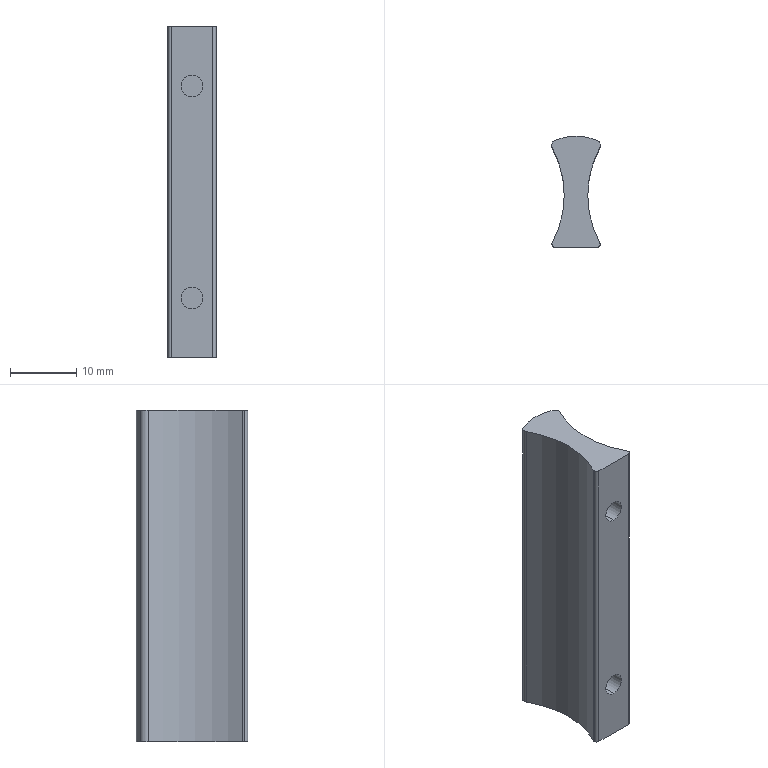Part | STEP file | TOPNIKE 1205 aluminium handle, hole spacing 32mm | 1 solid | 19 faces | box 7.369 x 16.8 x 50 mm | volume 4040 mm3 | cylinder 14 | plane 5 | commonest cylinder face diameters 3.3 x4 1 x3 1.6 x3 30 x3 16 x1
STEP:
#1=CARTESIAN_POINT('',(0.,0.,0.));
#2=DIRECTION('',(0.,0.,1.));
#3=DIRECTION('',(1.,0.,0.));
#4=AXIS2_PLACEMENT_3D('',#1,#2,#3);
#5=CARTESIAN_POINT('',(-3.634,-8.3,25.));
#6=VERTEX_POINT('',#5);
#7=CARTESIAN_POINT('',(-3.134,-8.8,25.));
#8=VERTEX_POINT('',#7);
#9=CARTESIAN_POINT('',(-3.134,-8.3,25.));
#10=DIRECTION('',(0.,0.,1.));
#11=DIRECTION('',(-1.,0.,0.));
#12=AXIS2_PLACEMENT_3D('',#9,#10,#11);
#13=CIRCLE('',#12,0.5);
#14=CARTESIAN_POINT('',(-3.134,-8.3,25.));
#15=DIRECTION('',(0.,0.,-1.));
#16=DIRECTION('',(-1.,0.,0.));
#17=AXIS2_PLACEMENT_3D('',#14,#15,#16);
#18=CYLINDRICAL_SURFACE('',#17,0.5);
#19=CARTESIAN_POINT('',(6.283,0.));
#20=DIRECTION('',(-1.,0.));
#21=VECTOR('',#20,1.);
#22=LINE('',#19,#21);
#23=(GEOMETRIC_REPRESENTATION_CONTEXT(2)PARAMETRIC_REPRESENTATION_CONTEXT()REPRESENTATION_CONTEXT('',''));
#24=DEFINITIONAL_REPRESENTATION('',(#22),#23);
#25=PCURVE('',#18,#24);
#26=CARTESIAN_POINT('',(-16.773,-0.9359,25.));
#27=DIRECTION('',(0.,0.,-1.));
#28=DIRECTION('',(-1.,0.,0.));
#29=AXIS2_PLACEMENT_3D('',#26,#27,#28);
#30=PLANE('',#29);
#31=CARTESIAN_POINT('',(-13.139,-7.364));
#32=CARTESIAN_POINT('',(-13.139,-8.23));
#33=CARTESIAN_POINT('',(-13.889,-7.797));
#34=CARTESIAN_POINT('',(-14.639,-7.364));
#35=CARTESIAN_POINT('',(-13.889,-6.931));
#36=CARTESIAN_POINT('',(-13.139,-6.498));
#37=CARTESIAN_POINT('',(-13.139,-7.364));
#38=(BOUNDED_CURVE()B_SPLINE_CURVE(2,(#31,#32,#33,#34,#35,#36,#37),.UNSPECIFIED.,.T.,.F.)B_SPLINE_CURVE_WITH_KNOTS((1,2,2,2,2,1),(-2.094,0.,2.094,4.189,6.283,8.378),.UNSPECIFIED.)CURVE()GEOMETRIC_REPRESENTATION_ITEM()RATIONAL_B_SPLINE_CURVE((1.,0.5,1.,0.5,1.,0.5,1.))REPRESENTATION_ITEM(''));
#39=(GEOMETRIC_REPRESENTATION_CONTEXT(2)PARAMETRIC_REPRESENTATION_CONTEXT()REPRESENTATION_CONTEXT('',''));
#40=DEFINITIONAL_REPRESENTATION('',(#38),#39);
#41=PCURVE('',#30,#40);
#42=SURFACE_CURVE('',#13,(#25,#41),.PCURVE_S1.);
#43=EDGE_CURVE('',#6,#8,#42,.T.);
#44=ORIENTED_EDGE('',*,*,#43,.F.);
#45=CARTESIAN_POINT('',(-3.634,-8.3,-25.));
#46=VERTEX_POINT('',#45);
#47=CARTESIAN_POINT('',(-3.634,-8.3,25.));
#48=DIRECTION('',(0.,0.,-1.));
#49=VECTOR('',#48,1.);
#50=LINE('',#47,#49);
#51=CARTESIAN_POINT('',(6.283,0.));
#52=DIRECTION('',(0.,1.));
#53=VECTOR('',#52,1.);
#54=LINE('',#51,#53);
#55=(GEOMETRIC_REPRESENTATION_CONTEXT(2)PARAMETRIC_REPRESENTATION_CONTEXT()REPRESENTATION_CONTEXT('',''));
#56=DEFINITIONAL_REPRESENTATION('',(#54),#55);
#57=PCURVE('',#18,#56);
#58=CARTESIAN_POINT('',(-3.134,-8.3,25.));
#59=DIRECTION('',(0.,0.,-1.));
#60=DIRECTION('',(-1.,0.,0.));
#61=AXIS2_PLACEMENT_3D('',#58,#59,#60);
#62=CYLINDRICAL_SURFACE('',#61,0.5);
#63=CARTESIAN_POINT('',(0.,0.));
#64=DIRECTION('',(0.,1.));
#65=VECTOR('',#64,1.);
#66=LINE('',#63,#65);
#67=(GEOMETRIC_REPRESENTATION_CONTEXT(2)PARAMETRIC_REPRESENTATION_CONTEXT()REPRESENTATION_CONTEXT('',''));
#68=DEFINITIONAL_REPRESENTATION('',(#66),#67);
#69=PCURVE('',#62,#68);
#70=SURFACE_CURVE('',#50,(#57,#69),.PCURVE_S1.);
#71=EDGE_CURVE('',#6,#46,#70,.T.);
#72=ORIENTED_EDGE('',*,*,#71,.T.);
#73=CARTESIAN_POINT('',(-3.134,-8.8,-25.));
#74=VERTEX_POINT('',#73);
#75=CARTESIAN_POINT('',(-3.134,-8.3,-25.));
#76=DIRECTION('',(0.,0.,-1.));
#77=DIRECTION('',(-1.,0.,0.));
#78=AXIS2_PLACEMENT_3D('',#75,#76,#77);
#79=CIRCLE('',#78,0.5);
#80=CARTESIAN_POINT('',(0.,50.));
#81=DIRECTION('',(1.,0.));
#82=VECTOR('',#81,1.);
#83=LINE('',#80,#82);
#84=(GEOMETRIC_REPRESENTATION_CONTEXT(2)PARAMETRIC_REPRESENTATION_CONTEXT()REPRESENTATION_CONTEXT('',''));
#85=DEFINITIONAL_REPRESENTATION('',(#83),#84);
#86=PCURVE('',#18,#85);
#87=CARTESIAN_POINT('',(-16.773,-0.9359,-25.));
#88=DIRECTION('',(0.,0.,-1.));
#89=DIRECTION('',(-1.,0.,0.));
#90=AXIS2_PLACEMENT_3D('',#87,#88,#89);
#91=PLANE('',#90);
#92=CARTESIAN_POINT('',(-13.639,-7.364));
#93=DIRECTION('',(1.,0.));
#94=AXIS2_PLACEMENT_2D('',#92,#93);
#95=CIRCLE('',#94,0.5);
#96=(GEOMETRIC_REPRESENTATION_CONTEXT(2)PARAMETRIC_REPRESENTATION_CONTEXT()REPRESENTATION_CONTEXT('',''));
#97=DEFINITIONAL_REPRESENTATION('',(#95),#96);
#98=PCURVE('',#91,#97);
#99=SURFACE_CURVE('',#79,(#86,#98),.PCURVE_S1.);
#100=EDGE_CURVE('',#74,#46,#99,.T.);
#101=ORIENTED_EDGE('',*,*,#100,.F.);
#102=CARTESIAN_POINT('',(-3.134,-8.8,25.));
#103=DIRECTION('',(0.,0.,-1.));
#104=VECTOR('',#103,1.);
#105=LINE('',#102,#104);
#106=CARTESIAN_POINT('',(4.712,0.));
#107=DIRECTION('',(0.,1.));
#108=VECTOR('',#107,1.);
#109=LINE('',#106,#108);
#110=(GEOMETRIC_REPRESENTATION_CONTEXT(2)PARAMETRIC_REPRESENTATION_CONTEXT()REPRESENTATION_CONTEXT('',''));
#111=DEFINITIONAL_REPRESENTATION('',(#109),#110);
#112=PCURVE('',#18,#111);
#113=CARTESIAN_POINT('',(4.,-8.8,25.));
#114=DIRECTION('',(0.,1.,0.));
#115=DIRECTION('',(0.,0.,1.));
#116=AXIS2_PLACEMENT_3D('',#113,#114,#115);
#117=PLANE('',#116);
#118=CARTESIAN_POINT('',(0.,-7.134));
#119=DIRECTION('',(-1.,0.));
#120=VECTOR('',#119,1.);
#121=LINE('',#118,#120);
#122=(GEOMETRIC_REPRESENTATION_CONTEXT(2)PARAMETRIC_REPRESENTATION_CONTEXT()REPRESENTATION_CONTEXT('',''));
#123=DEFINITIONAL_REPRESENTATION('',(#121),#122);
#124=PCURVE('',#117,#123);
#125=SURFACE_CURVE('',#105,(#112,#124),.PCURVE_S1.);
#126=EDGE_CURVE('',#8,#74,#125,.T.);
#127=ORIENTED_EDGE('',*,*,#126,.F.);
#128=EDGE_LOOP('',(#44,#72,#101,#127));
#129=FACE_BOUND('',#128,.T.);
#130=ADVANCED_FACE('',(#129),#18,.T.);
#131=CARTESIAN_POINT('',(3.685,6.597,-25.));
#132=VERTEX_POINT('',#131);
#133=CARTESIAN_POINT('',(3.588,6.216,-25.));
#134=VERTEX_POINT('',#133);
#135=CARTESIAN_POINT('',(2.885,6.597,-25.));
#136=DIRECTION('',(0.,0.,-1.));
#137=DIRECTION('',(-1.,0.,0.));
#138=AXIS2_PLACEMENT_3D('',#135,#136,#137);
#139=CIRCLE('',#138,0.8);
#140=CARTESIAN_POINT('',(2.885,6.597,25.));
#141=DIRECTION('',(0.,0.,1.));
#142=DIRECTION('',(1.,0.,0.));
#143=AXIS2_PLACEMENT_3D('',#140,#141,#142);
#144=CYLINDRICAL_SURFACE('',#143,0.8);
#145=CARTESIAN_POINT('',(9.425,-50.));
#146=DIRECTION('',(-1.,0.));
#147=VECTOR('',#146,1.);
#148=LINE('',#145,#147);
#149=(GEOMETRIC_REPRESENTATION_CONTEXT(2)PARAMETRIC_REPRESENTATION_CONTEXT()REPRESENTATION_CONTEXT('',''));
#150=DEFINITIONAL_REPRESENTATION('',(#148),#149);
#151=PCURVE('',#144,#150);
#152=CARTESIAN_POINT('',(-19.658,7.533));
#153=DIRECTION('',(1.,0.));
#154=AXIS2_PLACEMENT_2D('',#152,#153);
#155=CIRCLE('',#154,0.8);
#156=(GEOMETRIC_REPRESENTATION_CONTEXT(2)PARAMETRIC_REPRESENTATION_CONTEXT()REPRESENTATION_CONTEXT('',''));
#157=DEFINITIONAL_REPRESENTATION('',(#155),#156);
#158=PCURVE('',#91,#157);
#159=SURFACE_CURVE('',#139,(#151,#158),.PCURVE_S1.);
#160=EDGE_CURVE('',#132,#134,#159,.T.);
#161=ORIENTED_EDGE('',*,*,#160,.F.);
#162=CARTESIAN_POINT('',(3.685,6.597,25.));
#163=VERTEX_POINT('',#162);
#164=CARTESIAN_POINT('',(3.685,6.597,25.));
#165=DIRECTION('',(0.,0.,1.));
#166=VECTOR('',#165,1.);
#167=LINE('',#164,#166);
#168=CARTESIAN_POINT('',(6.283,0.));
#169=DIRECTION('',(0.,1.));
#170=VECTOR('',#169,1.);
#171=LINE('',#168,#170);
#172=(GEOMETRIC_REPRESENTATION_CONTEXT(2)PARAMETRIC_REPRESENTATION_CONTEXT()REPRESENTATION_CONTEXT('',''));
#173=DEFINITIONAL_REPRESENTATION('',(#171),#172);
#174=PCURVE('',#144,#173);
#175=CARTESIAN_POINT('',(2.885,6.597,25.));
#176=DIRECTION('',(0.,0.,1.));
#177=DIRECTION('',(1.,0.,0.));
#178=AXIS2_PLACEMENT_3D('',#175,#176,#177);
#179=CYLINDRICAL_SURFACE('',#178,0.8);
#180=CARTESIAN_POINT('',(0.,0.));
#181=DIRECTION('',(0.,1.));
#182=VECTOR('',#181,1.);
#183=LINE('',#180,#182);
#184=(GEOMETRIC_REPRESENTATION_CONTEXT(2)PARAMETRIC_REPRESENTATION_CONTEXT()REPRESENTATION_CONTEXT('',''));
#185=DEFINITIONAL_REPRESENTATION('',(#183),#184);
#186=PCURVE('',#179,#185);
#187=SURFACE_CURVE('',#167,(#174,#186),.PCURVE_S1.);
#188=EDGE_CURVE('',#132,#163,#187,.T.);
#189=ORIENTED_EDGE('',*,*,#188,.T.);
#190=CARTESIAN_POINT('',(3.588,6.216,25.));
#191=VERTEX_POINT('',#190);
#192=CARTESIAN_POINT('',(2.885,6.597,25.));
#193=DIRECTION('',(0.,0.,1.));
#194=DIRECTION('',(-1.,0.,0.));
#195=AXIS2_PLACEMENT_3D('',#192,#193,#194);
#196=CIRCLE('',#195,0.8);
#197=CARTESIAN_POINT('',(3.142,0.));
#198=DIRECTION('',(1.,0.));
#199=VECTOR('',#198,1.);
#200=LINE('',#197,#199);
#201=(GEOMETRIC_REPRESENTATION_CONTEXT(2)PARAMETRIC_REPRESENTATION_CONTEXT()REPRESENTATION_CONTEXT('',''));
#202=DEFINITIONAL_REPRESENTATION('',(#200),#201);
#203=PCURVE('',#144,#202);
#204=CARTESIAN_POINT('',(-18.858,7.533));
#205=CARTESIAN_POINT('',(-18.858,6.147));
#206=CARTESIAN_POINT('',(-20.058,6.84));
#207=CARTESIAN_POINT('',(-21.258,7.533));
#208=CARTESIAN_POINT('',(-20.058,8.226));
#209=CARTESIAN_POINT('',(-18.858,8.918));
#210=CARTESIAN_POINT('',(-18.858,7.533));
#211=(BOUNDED_CURVE()B_SPLINE_CURVE(2,(#204,#205,#206,#207,#208,#209,#210),.UNSPECIFIED.,.T.,.F.)B_SPLINE_CURVE_WITH_KNOTS((1,2,2,2,2,1),(-2.094,0.,2.094,4.189,6.283,8.378),.UNSPECIFIED.)CURVE()GEOMETRIC_REPRESENTATION_ITEM()RATIONAL_B_SPLINE_CURVE((1.,0.5,1.,0.5,1.,0.5,1.))REPRESENTATION_ITEM(''));
#212=(GEOMETRIC_REPRESENTATION_CONTEXT(2)PARAMETRIC_REPRESENTATION_CONTEXT()REPRESENTATION_CONTEXT('',''));
#213=DEFINITIONAL_REPRESENTATION('',(#211),#212);
#214=PCURVE('',#30,#213);
#215=SURFACE_CURVE('',#196,(#203,#214),.PCURVE_S1.);
#216=EDGE_CURVE('',#191,#163,#215,.T.);
#217=ORIENTED_EDGE('',*,*,#216,.F.);
#218=CARTESIAN_POINT('',(3.588,6.216,25.));
#219=DIRECTION('',(0.,0.,1.));
#220=VECTOR('',#219,1.);
#221=LINE('',#218,#220);
#222=CARTESIAN_POINT('',(5.786,0.));
#223=DIRECTION('',(0.,1.));
#224=VECTOR('',#223,1.);
#225=LINE('',#222,#224);
#226=(GEOMETRIC_REPRESENTATION_CONTEXT(2)PARAMETRIC_REPRESENTATION_CONTEXT()REPRESENTATION_CONTEXT('',''));
#227=DEFINITIONAL_REPRESENTATION('',(#225),#226);
#228=PCURVE('',#144,#227);
#229=CARTESIAN_POINT('',(16.773,-0.9359,25.));
#230=DIRECTION('',(0.,0.,-1.));
#231=DIRECTION('',(-1.,0.,0.));
#232=AXIS2_PLACEMENT_3D('',#229,#230,#231);
#233=CYLINDRICAL_SURFACE('',#232,15.);
#234=CARTESIAN_POINT('',(0.497,0.));
#235=DIRECTION('',(0.,-1.));
#236=VECTOR('',#235,1.);
#237=LINE('',#234,#236);
#238=(GEOMETRIC_REPRESENTATION_CONTEXT(2)PARAMETRIC_REPRESENTATION_CONTEXT()REPRESENTATION_CONTEXT('',''));
#239=DEFINITIONAL_REPRESENTATION('',(#237),#238);
#240=PCURVE('',#233,#239);
#241=SURFACE_CURVE('',#221,(#228,#240),.PCURVE_S1.);
#242=EDGE_CURVE('',#134,#191,#241,.T.);
#243=ORIENTED_EDGE('',*,*,#242,.F.);
#244=EDGE_LOOP('',(#161,#189,#217,#243));
#245=FACE_BOUND('',#244,.T.);
#246=ADVANCED_FACE('',(#245),#144,.T.);
#247=CARTESIAN_POINT('',(0.,-0.8,-17.65));
#248=VERTEX_POINT('',#247);
#249=CARTESIAN_POINT('',(0.,-8.8,-17.65));
#250=VERTEX_POINT('',#249);
#251=CARTESIAN_POINT('',(0.,-0.8,-17.65));
#252=DIRECTION('',(0.,-1.,0.));
#253=VECTOR('',#252,1.);
#254=LINE('',#251,#253);
#255=CARTESIAN_POINT('',(0.,-0.8,-16.));
#256=DIRECTION('',(0.,-1.,0.));
#257=DIRECTION('',(0.,0.,-1.));
#258=AXIS2_PLACEMENT_3D('',#255,#256,#257);
#259=CYLINDRICAL_SURFACE('',#258,1.65);
#260=CARTESIAN_POINT('',(6.283,0.));
#261=DIRECTION('',(0.,1.));
#262=VECTOR('',#261,1.);
#263=LINE('',#260,#262);
#264=(GEOMETRIC_REPRESENTATION_CONTEXT(2)PARAMETRIC_REPRESENTATION_CONTEXT()REPRESENTATION_CONTEXT('',''));
#265=DEFINITIONAL_REPRESENTATION('',(#263),#264);
#266=PCURVE('',#259,#265);
#267=CARTESIAN_POINT('',(0.,-0.8,-16.));
#268=DIRECTION('',(0.,-1.,0.));
#269=DIRECTION('',(0.,0.,-1.));
#270=AXIS2_PLACEMENT_3D('',#267,#268,#269);
#271=CYLINDRICAL_SURFACE('',#270,1.65);
#272=CARTESIAN_POINT('',(0.,0.));
#273=DIRECTION('',(0.,1.));
#274=VECTOR('',#273,1.);
#275=LINE('',#272,#274);
#276=(GEOMETRIC_REPRESENTATION_CONTEXT(2)PARAMETRIC_REPRESENTATION_CONTEXT()REPRESENTATION_CONTEXT('',''));
#277=DEFINITIONAL_REPRESENTATION('',(#275),#276);
#278=PCURVE('',#271,#277);
#279=SURFACE_CURVE('',#254,(#266,#278),.PCURVE_S1.);
#280=EDGE_CURVE('',#248,#250,#279,.T.);
#281=ORIENTED_EDGE('',*,*,#280,.T.);
#282=CARTESIAN_POINT('',(0.,-8.8,-14.35));
#283=VERTEX_POINT('',#282);
#284=CARTESIAN_POINT('',(0.,-8.8,-16.));
#285=DIRECTION('',(0.,-1.,0.));
#286=DIRECTION('',(0.,0.,-1.));
#287=AXIS2_PLACEMENT_3D('',#284,#285,#286);
#288=CIRCLE('',#287,1.65);
#289=CARTESIAN_POINT('',(0.,8.));
#290=DIRECTION('',(1.,0.));
#291=VECTOR('',#290,1.);
#292=LINE('',#289,#291);
#293=(GEOMETRIC_REPRESENTATION_CONTEXT(2)PARAMETRIC_REPRESENTATION_CONTEXT()REPRESENTATION_CONTEXT('',''));
#294=DEFINITIONAL_REPRESENTATION('',(#292),#293);
#295=PCURVE('',#259,#294);
#296=CARTESIAN_POINT('',(-42.65,-4.));
#297=CARTESIAN_POINT('',(-42.65,-1.142));
#298=CARTESIAN_POINT('',(-40.175,-2.571));
#299=CARTESIAN_POINT('',(-37.7,-4.));
#300=CARTESIAN_POINT('',(-40.175,-5.429));
#301=CARTESIAN_POINT('',(-42.65,-6.858));
#302=CARTESIAN_POINT('',(-42.65,-4.));
#303=(BOUNDED_CURVE()B_SPLINE_CURVE(2,(#296,#297,#298,#299,#300,#301,#302),.UNSPECIFIED.,.T.,.F.)B_SPLINE_CURVE_WITH_KNOTS((1,2,2,2,2,1),(-2.094,0.,2.094,4.189,6.283,8.378),.UNSPECIFIED.)CURVE()GEOMETRIC_REPRESENTATION_ITEM()RATIONAL_B_SPLINE_CURVE((1.,0.5,1.,0.5,1.,0.5,1.))REPRESENTATION_ITEM(''));
#304=(GEOMETRIC_REPRESENTATION_CONTEXT(2)PARAMETRIC_REPRESENTATION_CONTEXT()REPRESENTATION_CONTEXT('',''));
#305=DEFINITIONAL_REPRESENTATION('',(#303),#304);
#306=PCURVE('',#117,#305);
#307=SURFACE_CURVE('',#288,(#295,#306),.PCURVE_S1.);
#308=EDGE_CURVE('',#283,#250,#307,.T.);
#309=ORIENTED_EDGE('',*,*,#308,.F.);
#310=CARTESIAN_POINT('',(0.,-0.8,-14.35));
#311=VERTEX_POINT('',#310);
#312=CARTESIAN_POINT('',(0.,-0.8,-14.35));
#313=DIRECTION('',(0.,-1.,0.));
#314=VECTOR('',#313,1.);
#315=LINE('',#312,#314);
#316=CARTESIAN_POINT('',(3.142,0.));
#317=DIRECTION('',(0.,1.));
#318=VECTOR('',#317,1.);
#319=LINE('',#316,#318);
#320=(GEOMETRIC_REPRESENTATION_CONTEXT(2)PARAMETRIC_REPRESENTATION_CONTEXT()REPRESENTATION_CONTEXT('',''));
#321=DEFINITIONAL_REPRESENTATION('',(#319),#320);
#322=PCURVE('',#259,#321);
#323=CARTESIAN_POINT('',(3.142,0.));
#324=DIRECTION('',(0.,1.));
#325=VECTOR('',#324,1.);
#326=LINE('',#323,#325);
#327=(GEOMETRIC_REPRESENTATION_CONTEXT(2)PARAMETRIC_REPRESENTATION_CONTEXT()REPRESENTATION_CONTEXT('',''));
#328=DEFINITIONAL_REPRESENTATION('',(#326),#327);
#329=PCURVE('',#271,#328);
#330=SURFACE_CURVE('',#315,(#322,#329),.PCURVE_S1.);
#331=EDGE_CURVE('',#311,#283,#330,.T.);
#332=ORIENTED_EDGE('',*,*,#331,.F.);
#333=CARTESIAN_POINT('',(0.,-0.8,-16.));
#334=DIRECTION('',(0.,-1.,0.));
#335=DIRECTION('',(0.,0.,-1.));
#336=AXIS2_PLACEMENT_3D('',#333,#334,#335);
#337=CIRCLE('',#336,1.65);
#338=CARTESIAN_POINT('',(0.,0.));
#339=DIRECTION('',(1.,0.));
#340=VECTOR('',#339,1.);
#341=LINE('',#338,#340);
#342=(GEOMETRIC_REPRESENTATION_CONTEXT(2)PARAMETRIC_REPRESENTATION_CONTEXT()REPRESENTATION_CONTEXT('',''));
#343=DEFINITIONAL_REPRESENTATION('',(#341),#342);
#344=PCURVE('',#259,#343);
#345=CARTESIAN_POINT('',(0.,-0.8,-16.));
#346=DIRECTION('',(0.,-1.,0.));
#347=DIRECTION('',(0.,0.,-1.));
#348=AXIS2_PLACEMENT_3D('',#345,#346,#347);
#349=PLANE('',#348);
#350=CARTESIAN_POINT('',(0.,0.));
#351=DIRECTION('',(1.,0.));
#352=AXIS2_PLACEMENT_2D('',#350,#351);
#353=CIRCLE('',#352,1.65);
#354=(GEOMETRIC_REPRESENTATION_CONTEXT(2)PARAMETRIC_REPRESENTATION_CONTEXT()REPRESENTATION_CONTEXT('',''));
#355=DEFINITIONAL_REPRESENTATION('',(#353),#354);
#356=PCURVE('',#349,#355);
#357=SURFACE_CURVE('',#337,(#344,#356),.PCURVE_S1.);
#358=EDGE_CURVE('',#311,#248,#357,.T.);
#359=ORIENTED_EDGE('',*,*,#358,.T.);
#360=EDGE_LOOP('',(#281,#309,#332,#359));
#361=FACE_BOUND('',#360,.F.);
#362=ADVANCED_FACE('',(#361),#259,.F.);
#363=CARTESIAN_POINT('',(0.,-0.8,14.35));
#364=VERTEX_POINT('',#363);
#365=CARTESIAN_POINT('',(0.,-8.8,14.35));
#366=VERTEX_POINT('',#365);
#367=CARTESIAN_POINT('',(0.,-0.8,14.35));
#368=DIRECTION('',(0.,-1.,0.));
#369=VECTOR('',#368,1.);
#370=LINE('',#367,#369);
#371=CARTESIAN_POINT('',(0.,-0.8,16.));
#372=DIRECTION('',(0.,-1.,0.));
#373=DIRECTION('',(0.,0.,-1.));
#374=AXIS2_PLACEMENT_3D('',#371,#372,#373);
#375=CYLINDRICAL_SURFACE('',#374,1.65);
#376=CARTESIAN_POINT('',(6.283,0.));
#377=DIRECTION('',(0.,1.));
#378=VECTOR('',#377,1.);
#379=LINE('',#376,#378);
#380=(GEOMETRIC_REPRESENTATION_CONTEXT(2)PARAMETRIC_REPRESENTATION_CONTEXT()REPRESENTATION_CONTEXT('',''));
#381=DEFINITIONAL_REPRESENTATION('',(#379),#380);
#382=PCURVE('',#375,#381);
#383=CARTESIAN_POINT('',(0.,-0.8,16.));
#384=DIRECTION('',(0.,-1.,0.));
#385=DIRECTION('',(0.,0.,-1.));
#386=AXIS2_PLACEMENT_3D('',#383,#384,#385);
#387=CYLINDRICAL_SURFACE('',#386,1.65);
#388=CARTESIAN_POINT('',(0.,0.));
#389=DIRECTION('',(0.,1.));
#390=VECTOR('',#389,1.);
#391=LINE('',#388,#390);
#392=(GEOMETRIC_REPRESENTATION_CONTEXT(2)PARAMETRIC_REPRESENTATION_CONTEXT()REPRESENTATION_CONTEXT('',''));
#393=DEFINITIONAL_REPRESENTATION('',(#391),#392);
#394=PCURVE('',#387,#393);
#395=SURFACE_CURVE('',#370,(#382,#394),.PCURVE_S1.);
#396=EDGE_CURVE('',#364,#366,#395,.T.);
#397=ORIENTED_EDGE('',*,*,#396,.T.);
#398=CARTESIAN_POINT('',(0.,-8.8,17.65));
#399=VERTEX_POINT('',#398);
#400=CARTESIAN_POINT('',(0.,-8.8,16.));
#401=DIRECTION('',(0.,-1.,0.));
#402=DIRECTION('',(0.,0.,-1.));
#403=AXIS2_PLACEMENT_3D('',#400,#401,#402);
#404=CIRCLE('',#403,1.65);
#405=CARTESIAN_POINT('',(0.,8.));
#406=DIRECTION('',(1.,0.));
#407=VECTOR('',#406,1.);
#408=LINE('',#405,#407);
#409=(GEOMETRIC_REPRESENTATION_CONTEXT(2)PARAMETRIC_REPRESENTATION_CONTEXT()REPRESENTATION_CONTEXT('',''));
#410=DEFINITIONAL_REPRESENTATION('',(#408),#409);
#411=PCURVE('',#375,#410);
#412=CARTESIAN_POINT('',(-10.65,-4.));
#413=CARTESIAN_POINT('',(-10.65,-1.142));
#414=CARTESIAN_POINT('',(-8.175,-2.571));
#415=CARTESIAN_POINT('',(-5.7,-4.));
#416=CARTESIAN_POINT('',(-8.175,-5.429));
#417=CARTESIAN_POINT('',(-10.65,-6.858));
#418=CARTESIAN_POINT('',(-10.65,-4.));
#419=(BOUNDED_CURVE()B_SPLINE_CURVE(2,(#412,#413,#414,#415,#416,#417,#418),.UNSPECIFIED.,.T.,.F.)B_SPLINE_CURVE_WITH_KNOTS((1,2,2,2,2,1),(-2.094,0.,2.094,4.189,6.283,8.378),.UNSPECIFIED.)CURVE()GEOMETRIC_REPRESENTATION_ITEM()RATIONAL_B_SPLINE_CURVE((1.,0.5,1.,0.5,1.,0.5,1.))REPRESENTATION_ITEM(''));
#420=(GEOMETRIC_REPRESENTATION_CONTEXT(2)PARAMETRIC_REPRESENTATION_CONTEXT()REPRESENTATION_CONTEXT('',''));
#421=DEFINITIONAL_REPRESENTATION('',(#419),#420);
#422=PCURVE('',#117,#421);
#423=SURFACE_CURVE('',#404,(#411,#422),.PCURVE_S1.);
#424=EDGE_CURVE('',#399,#366,#423,.T.);
#425=ORIENTED_EDGE('',*,*,#424,.F.);
#426=CARTESIAN_POINT('',(0.,-0.8,17.65));
#427=VERTEX_POINT('',#426);
#428=CARTESIAN_POINT('',(0.,-0.8,17.65));
#429=DIRECTION('',(0.,-1.,0.));
#430=VECTOR('',#429,1.);
#431=LINE('',#428,#430);
#432=CARTESIAN_POINT('',(3.142,0.));
#433=DIRECTION('',(0.,1.));
#434=VECTOR('',#433,1.);
#435=LINE('',#432,#434);
#436=(GEOMETRIC_REPRESENTATION_CONTEXT(2)PARAMETRIC_REPRESENTATION_CONTEXT()REPRESENTATION_CONTEXT('',''));
#437=DEFINITIONAL_REPRESENTATION('',(#435),#436);
#438=PCURVE('',#375,#437);
#439=CARTESIAN_POINT('',(3.142,0.));
#440=DIRECTION('',(0.,1.));
#441=VECTOR('',#440,1.);
#442=LINE('',#439,#441);
#443=(GEOMETRIC_REPRESENTATION_CONTEXT(2)PARAMETRIC_REPRESENTATION_CONTEXT()REPRESENTATION_CONTEXT('',''));
#444=DEFINITIONAL_REPRESENTATION('',(#442),#443);
#445=PCURVE('',#387,#444);
#446=SURFACE_CURVE('',#431,(#438,#445),.PCURVE_S1.);
#447=EDGE_CURVE('',#427,#399,#446,.T.);
#448=ORIENTED_EDGE('',*,*,#447,.F.);
#449=CARTESIAN_POINT('',(0.,-0.8,16.));
#450=DIRECTION('',(0.,-1.,0.));
#451=DIRECTION('',(0.,0.,-1.));
#452=AXIS2_PLACEMENT_3D('',#449,#450,#451);
#453=CIRCLE('',#452,1.65);
#454=CARTESIAN_POINT('',(0.,0.));
#455=DIRECTION('',(1.,0.));
#456=VECTOR('',#455,1.);
#457=LINE('',#454,#456);
#458=(GEOMETRIC_REPRESENTATION_CONTEXT(2)PARAMETRIC_REPRESENTATION_CONTEXT()REPRESENTATION_CONTEXT('',''));
#459=DEFINITIONAL_REPRESENTATION('',(#457),#458);
#460=PCURVE('',#375,#459);
#461=CARTESIAN_POINT('',(0.,-0.8,16.));
#462=DIRECTION('',(0.,-1.,0.));
#463=DIRECTION('',(0.,0.,-1.));
#464=AXIS2_PLACEMENT_3D('',#461,#462,#463);
#465=PLANE('',#464);
#466=CARTESIAN_POINT('',(0.,0.));
#467=DIRECTION('',(1.,0.));
#468=AXIS2_PLACEMENT_2D('',#466,#467);
#469=CIRCLE('',#468,1.65);
#470=(GEOMETRIC_REPRESENTATION_CONTEXT(2)PARAMETRIC_REPRESENTATION_CONTEXT()REPRESENTATION_CONTEXT('',''));
#471=DEFINITIONAL_REPRESENTATION('',(#469),#470);
#472=PCURVE('',#465,#471);
#473=SURFACE_CURVE('',#453,(#460,#472),.PCURVE_S1.);
#474=EDGE_CURVE('',#427,#364,#473,.T.);
#475=ORIENTED_EDGE('',*,*,#474,.T.);
#476=EDGE_LOOP('',(#397,#425,#448,#475));
#477=FACE_BOUND('',#476,.F.);
#478=ADVANCED_FACE('',(#477),#375,.F.);
#479=ORIENTED_EDGE('',*,*,#242,.F.);
#480=CARTESIAN_POINT('',(1.773,-0.9359,-25.));
#481=VERTEX_POINT('',#480);
#482=CARTESIAN_POINT('',(16.773,-0.9359,-25.));
#483=DIRECTION('',(0.,0.,-1.));
#484=DIRECTION('',(1.,0.,0.));
#485=AXIS2_PLACEMENT_3D('',#482,#483,#484);
#486=CIRCLE('',#485,15.);
#487=CARTESIAN_POINT('',(-3.142,50.));
#488=DIRECTION('',(1.,0.));
#489=VECTOR('',#488,1.);
#490=LINE('',#487,#489);
#491=(GEOMETRIC_REPRESENTATION_CONTEXT(2)PARAMETRIC_REPRESENTATION_CONTEXT()REPRESENTATION_CONTEXT('',''));
#492=DEFINITIONAL_REPRESENTATION('',(#490),#491);
#493=PCURVE('',#233,#492);
#494=CARTESIAN_POINT('',(-33.546,0.));
#495=DIRECTION('',(-1.,0.));
#496=AXIS2_PLACEMENT_2D('',#494,#495);
#497=CIRCLE('',#496,15.);
#498=(GEOMETRIC_REPRESENTATION_CONTEXT(2)PARAMETRIC_REPRESENTATION_CONTEXT()REPRESENTATION_CONTEXT('',''));
#499=DEFINITIONAL_REPRESENTATION('',(#497),#498);
#500=PCURVE('',#91,#499);
#501=SURFACE_CURVE('',#486,(#493,#500),.PCURVE_S1.);
#502=EDGE_CURVE('',#481,#134,#501,.T.);
#503=ORIENTED_EDGE('',*,*,#502,.F.);
#504=CARTESIAN_POINT('',(1.773,-0.9359,25.));
#505=VERTEX_POINT('',#504);
#506=CARTESIAN_POINT('',(1.773,-0.9359,25.));
#507=DIRECTION('',(0.,0.,-1.));
#508=VECTOR('',#507,1.);
#509=LINE('',#506,#508);
#510=CARTESIAN_POINT('',(0.,0.));
#511=DIRECTION('',(0.,1.));
#512=VECTOR('',#511,1.);
#513=LINE('',#510,#512);
#514=(GEOMETRIC_REPRESENTATION_CONTEXT(2)PARAMETRIC_REPRESENTATION_CONTEXT()REPRESENTATION_CONTEXT('',''));
#515=DEFINITIONAL_REPRESENTATION('',(#513),#514);
#516=PCURVE('',#233,#515);
#517=CARTESIAN_POINT('',(16.773,-0.9359,25.));
#518=DIRECTION('',(0.,0.,-1.));
#519=DIRECTION('',(-1.,0.,0.));
#520=AXIS2_PLACEMENT_3D('',#517,#518,#519);
#521=CYLINDRICAL_SURFACE('',#520,15.);
#522=CARTESIAN_POINT('',(6.283,0.));
#523=DIRECTION('',(0.,1.));
#524=VECTOR('',#523,1.);
#525=LINE('',#522,#524);
#526=(GEOMETRIC_REPRESENTATION_CONTEXT(2)PARAMETRIC_REPRESENTATION_CONTEXT()REPRESENTATION_CONTEXT('',''));
#527=DEFINITIONAL_REPRESENTATION('',(#525),#526);
#528=PCURVE('',#521,#527);
#529=SURFACE_CURVE('',#509,(#516,#528),.PCURVE_S1.);
#530=EDGE_CURVE('',#505,#481,#529,.T.);
#531=ORIENTED_EDGE('',*,*,#530,.F.);
#532=CARTESIAN_POINT('',(16.773,-0.9359,25.));
#533=DIRECTION('',(0.,0.,-1.));
#534=DIRECTION('',(1.,0.,0.));
#535=AXIS2_PLACEMENT_3D('',#532,#533,#534);
#536=CIRCLE('',#535,15.);
#537=CARTESIAN_POINT('',(-3.142,0.));
#538=DIRECTION('',(1.,0.));
#539=VECTOR('',#538,1.);
#540=LINE('',#537,#539);
#541=(GEOMETRIC_REPRESENTATION_CONTEXT(2)PARAMETRIC_REPRESENTATION_CONTEXT()REPRESENTATION_CONTEXT('',''));
#542=DEFINITIONAL_REPRESENTATION('',(#540),#541);
#543=PCURVE('',#233,#542);
#544=CARTESIAN_POINT('',(-33.546,0.));
#545=DIRECTION('',(-1.,0.));
#546=AXIS2_PLACEMENT_2D('',#544,#545);
#547=CIRCLE('',#546,15.);
#548=(GEOMETRIC_REPRESENTATION_CONTEXT(2)PARAMETRIC_REPRESENTATION_CONTEXT()REPRESENTATION_CONTEXT('',''));
#549=DEFINITIONAL_REPRESENTATION('',(#547),#548);
#550=PCURVE('',#30,#549);
#551=SURFACE_CURVE('',#536,(#543,#550),.PCURVE_S1.);
#552=EDGE_CURVE('',#505,#191,#551,.T.);
#553=ORIENTED_EDGE('',*,*,#552,.T.);
#554=EDGE_LOOP('',(#479,#503,#531,#553));
#555=FACE_BOUND('',#554,.F.);
#556=ADVANCED_FACE('',(#555),#233,.F.);
#557=CARTESIAN_POINT('',(-3.588,6.216,25.));
#558=VERTEX_POINT('',#557);
#559=CARTESIAN_POINT('',(-3.588,6.216,-25.));
#560=VERTEX_POINT('',#559);
#561=CARTESIAN_POINT('',(-3.588,6.216,25.));
#562=DIRECTION('',(0.,0.,-1.));
#563=VECTOR('',#562,1.);
#564=LINE('',#561,#563);
#565=CARTESIAN_POINT('',(-16.773,-0.9359,25.));
#566=DIRECTION('',(0.,0.,-1.));
#567=DIRECTION('',(-1.,0.,0.));
#568=AXIS2_PLACEMENT_3D('',#565,#566,#567);
#569=CYLINDRICAL_SURFACE('',#568,15.);
#570=CARTESIAN_POINT('',(2.645,0.));
#571=DIRECTION('',(0.,1.));
#572=VECTOR('',#571,1.);
#573=LINE('',#570,#572);
#574=(GEOMETRIC_REPRESENTATION_CONTEXT(2)PARAMETRIC_REPRESENTATION_CONTEXT()REPRESENTATION_CONTEXT('',''));
#575=DEFINITIONAL_REPRESENTATION('',(#573),#574);
#576=PCURVE('',#569,#575);
#577=CARTESIAN_POINT('',(-2.885,6.597,25.));
#578=DIRECTION('',(0.,0.,1.));
#579=DIRECTION('',(1.,0.,0.));
#580=AXIS2_PLACEMENT_3D('',#577,#578,#579);
#581=CYLINDRICAL_SURFACE('',#580,0.8);
#582=CARTESIAN_POINT('',(3.639,0.));
#583=DIRECTION('',(0.,-1.));
#584=VECTOR('',#583,1.);
#585=LINE('',#582,#584);
#586=(GEOMETRIC_REPRESENTATION_CONTEXT(2)PARAMETRIC_REPRESENTATION_CONTEXT()REPRESENTATION_CONTEXT('',''));
#587=DEFINITIONAL_REPRESENTATION('',(#585),#586);
#588=PCURVE('',#581,#587);
#589=SURFACE_CURVE('',#564,(#576,#588),.PCURVE_S1.);
#590=EDGE_CURVE('',#558,#560,#589,.T.);
#591=ORIENTED_EDGE('',*,*,#590,.F.);
#592=CARTESIAN_POINT('',(-3.574,-8.062,25.));
#593=VERTEX_POINT('',#592);
#594=CARTESIAN_POINT('',(-16.773,-0.9359,25.));
#595=DIRECTION('',(0.,0.,-1.));
#596=DIRECTION('',(-1.,0.,0.));
#597=AXIS2_PLACEMENT_3D('',#594,#595,#596);
#598=CIRCLE('',#597,15.);
#599=CARTESIAN_POINT('',(0.,0.));
#600=DIRECTION('',(1.,0.));
#601=VECTOR('',#600,1.);
#602=LINE('',#599,#601);
#603=(GEOMETRIC_REPRESENTATION_CONTEXT(2)PARAMETRIC_REPRESENTATION_CONTEXT()REPRESENTATION_CONTEXT('',''));
#604=DEFINITIONAL_REPRESENTATION('',(#602),#603);
#605=PCURVE('',#569,#604);
#606=CARTESIAN_POINT('',(0.,0.));
#607=DIRECTION('',(1.,0.));
#608=AXIS2_PLACEMENT_2D('',#606,#607);
#609=CIRCLE('',#608,15.);
#610=(GEOMETRIC_REPRESENTATION_CONTEXT(2)PARAMETRIC_REPRESENTATION_CONTEXT()REPRESENTATION_CONTEXT('',''));
#611=DEFINITIONAL_REPRESENTATION('',(#609),#610);
#612=PCURVE('',#30,#611);
#613=SURFACE_CURVE('',#598,(#605,#612),.PCURVE_S1.);
#614=EDGE_CURVE('',#558,#593,#613,.T.);
#615=ORIENTED_EDGE('',*,*,#614,.T.);
#616=CARTESIAN_POINT('',(-3.574,-8.062,-25.));
#617=VERTEX_POINT('',#616);
#618=CARTESIAN_POINT('',(-3.574,-8.062,25.));
#619=DIRECTION('',(0.,0.,1.));
#620=VECTOR('',#619,1.);
#621=LINE('',#618,#620);
#622=CARTESIAN_POINT('',(3.637,0.));
#623=DIRECTION('',(0.,-1.));
#624=VECTOR('',#623,1.);
#625=LINE('',#622,#624);
#626=(GEOMETRIC_REPRESENTATION_CONTEXT(2)PARAMETRIC_REPRESENTATION_CONTEXT()REPRESENTATION_CONTEXT('',''));
#627=DEFINITIONAL_REPRESENTATION('',(#625),#626);
#628=PCURVE('',#569,#627);
#629=CARTESIAN_POINT('',(0.4951,0.));
#630=DIRECTION('',(0.,-1.));
#631=VECTOR('',#630,1.);
#632=LINE('',#629,#631);
#633=(GEOMETRIC_REPRESENTATION_CONTEXT(2)PARAMETRIC_REPRESENTATION_CONTEXT()REPRESENTATION_CONTEXT('',''));
#634=DEFINITIONAL_REPRESENTATION('',(#632),#633);
#635=PCURVE('',#62,#634);
#636=SURFACE_CURVE('',#621,(#628,#635),.PCURVE_S1.);
#637=EDGE_CURVE('',#617,#593,#636,.T.);
#638=ORIENTED_EDGE('',*,*,#637,.F.);
#639=CARTESIAN_POINT('',(-16.773,-0.9359,-25.));
#640=DIRECTION('',(0.,0.,-1.));
#641=DIRECTION('',(-1.,0.,0.));
#642=AXIS2_PLACEMENT_3D('',#639,#640,#641);
#643=CIRCLE('',#642,15.);
#644=CARTESIAN_POINT('',(0.,50.));
#645=DIRECTION('',(1.,0.));
#646=VECTOR('',#645,1.);
#647=LINE('',#644,#646);
#648=(GEOMETRIC_REPRESENTATION_CONTEXT(2)PARAMETRIC_REPRESENTATION_CONTEXT()REPRESENTATION_CONTEXT('',''));
#649=DEFINITIONAL_REPRESENTATION('',(#647),#648);
#650=PCURVE('',#569,#649);
#651=CARTESIAN_POINT('',(0.,0.));
#652=DIRECTION('',(1.,0.));
#653=AXIS2_PLACEMENT_2D('',#651,#652);
#654=CIRCLE('',#653,15.);
#655=(GEOMETRIC_REPRESENTATION_CONTEXT(2)PARAMETRIC_REPRESENTATION_CONTEXT()REPRESENTATION_CONTEXT('',''));
#656=DEFINITIONAL_REPRESENTATION('',(#654),#655);
#657=PCURVE('',#91,#656);
#658=SURFACE_CURVE('',#643,(#650,#657),.PCURVE_S1.);
#659=EDGE_CURVE('',#560,#617,#658,.T.);
#660=ORIENTED_EDGE('',*,*,#659,.F.);
#661=EDGE_LOOP('',(#591,#615,#638,#660));
#662=FACE_BOUND('',#661,.F.);
#663=ADVANCED_FACE('',(#662),#569,.F.);
#664=CARTESIAN_POINT('',(0.,-8.8,-16.));
#665=DIRECTION('',(0.,-1.,0.));
#666=DIRECTION('',(0.,0.,-1.));
#667=AXIS2_PLACEMENT_3D('',#664,#665,#666);
#668=CIRCLE('',#667,1.65);
#669=CARTESIAN_POINT('',(-42.65,-4.));
#670=CARTESIAN_POINT('',(-42.65,-1.142));
#671=CARTESIAN_POINT('',(-40.175,-2.571));
#672=CARTESIAN_POINT('',(-37.7,-4.));
#673=CARTESIAN_POINT('',(-40.175,-5.429));
#674=CARTESIAN_POINT('',(-42.65,-6.858));
#675=CARTESIAN_POINT('',(-42.65,-4.));
#676=(BOUNDED_CURVE()B_SPLINE_CURVE(2,(#669,#670,#671,#672,#673,#674,#675),.UNSPECIFIED.,.T.,.F.)B_SPLINE_CURVE_WITH_KNOTS((1,2,2,2,2,1),(-2.094,0.,2.094,4.189,6.283,8.378),.UNSPECIFIED.)CURVE()GEOMETRIC_REPRESENTATION_ITEM()RATIONAL_B_SPLINE_CURVE((1.,0.5,1.,0.5,1.,0.5,1.))REPRESENTATION_ITEM(''));
#677=(GEOMETRIC_REPRESENTATION_CONTEXT(2)PARAMETRIC_REPRESENTATION_CONTEXT()REPRESENTATION_CONTEXT('',''));
#678=DEFINITIONAL_REPRESENTATION('',(#676),#677);
#679=PCURVE('',#117,#678);
#680=CARTESIAN_POINT('',(0.,8.));
#681=DIRECTION('',(1.,0.));
#682=VECTOR('',#681,1.);
#683=LINE('',#680,#682);
#684=(GEOMETRIC_REPRESENTATION_CONTEXT(2)PARAMETRIC_REPRESENTATION_CONTEXT()REPRESENTATION_CONTEXT('',''));
#685=DEFINITIONAL_REPRESENTATION('',(#683),#684);
#686=PCURVE('',#271,#685);
#687=SURFACE_CURVE('',#668,(#679,#686),.PCURVE_S1.);
#688=EDGE_CURVE('',#250,#283,#687,.T.);
#689=ORIENTED_EDGE('',*,*,#688,.F.);
#690=ORIENTED_EDGE('',*,*,#308,.F.);
#691=EDGE_LOOP('',(#689,#690));
#692=FACE_BOUND('',#691,.T.);
#693=CARTESIAN_POINT('',(0.,-8.8,16.));
#694=DIRECTION('',(0.,-1.,0.));
#695=DIRECTION('',(0.,0.,-1.));
#696=AXIS2_PLACEMENT_3D('',#693,#694,#695);
#697=CIRCLE('',#696,1.65);
#698=CARTESIAN_POINT('',(-10.65,-4.));
#699=CARTESIAN_POINT('',(-10.65,-1.142));
#700=CARTESIAN_POINT('',(-8.175,-2.571));
#701=CARTESIAN_POINT('',(-5.7,-4.));
#702=CARTESIAN_POINT('',(-8.175,-5.429));
#703=CARTESIAN_POINT('',(-10.65,-6.858));
#704=CARTESIAN_POINT('',(-10.65,-4.));
#705=(BOUNDED_CURVE()B_SPLINE_CURVE(2,(#698,#699,#700,#701,#702,#703,#704),.UNSPECIFIED.,.T.,.F.)B_SPLINE_CURVE_WITH_KNOTS((1,2,2,2,2,1),(-2.094,0.,2.094,4.189,6.283,8.378),.UNSPECIFIED.)CURVE()GEOMETRIC_REPRESENTATION_ITEM()RATIONAL_B_SPLINE_CURVE((1.,0.5,1.,0.5,1.,0.5,1.))REPRESENTATION_ITEM(''));
#706=(GEOMETRIC_REPRESENTATION_CONTEXT(2)PARAMETRIC_REPRESENTATION_CONTEXT()REPRESENTATION_CONTEXT('',''));
#707=DEFINITIONAL_REPRESENTATION('',(#705),#706);
#708=PCURVE('',#117,#707);
#709=CARTESIAN_POINT('',(0.,8.));
#710=DIRECTION('',(1.,0.));
#711=VECTOR('',#710,1.);
#712=LINE('',#709,#711);
#713=(GEOMETRIC_REPRESENTATION_CONTEXT(2)PARAMETRIC_REPRESENTATION_CONTEXT()REPRESENTATION_CONTEXT('',''));
#714=DEFINITIONAL_REPRESENTATION('',(#712),#713);
#715=PCURVE('',#387,#714);
#716=SURFACE_CURVE('',#697,(#708,#715),.PCURVE_S1.);
#717=EDGE_CURVE('',#366,#399,#716,.T.);
#718=ORIENTED_EDGE('',*,*,#717,.F.);
#719=ORIENTED_EDGE('',*,*,#424,.F.);
#720=EDGE_LOOP('',(#718,#719));
#721=FACE_BOUND('',#720,.T.);
#722=CARTESIAN_POINT('',(3.134,-8.8,-25.));
#723=VERTEX_POINT('',#722);
#724=CARTESIAN_POINT('',(4.,-8.8,-25.));
#725=DIRECTION('',(1.,0.,0.));
#726=VECTOR('',#725,1.);
#727=LINE('',#724,#726);
#728=CARTESIAN_POINT('',(-50.,0.));
#729=DIRECTION('',(0.,1.));
#730=VECTOR('',#729,1.);
#731=LINE('',#728,#730);
#732=(GEOMETRIC_REPRESENTATION_CONTEXT(2)PARAMETRIC_REPRESENTATION_CONTEXT()REPRESENTATION_CONTEXT('',''));
#733=DEFINITIONAL_REPRESENTATION('',(#731),#732);
#734=PCURVE('',#117,#733);
#735=CARTESIAN_POINT('',(-20.773,-7.864));
#736=DIRECTION('',(-1.,0.));
#737=VECTOR('',#736,1.);
#738=LINE('',#735,#737);
#739=(GEOMETRIC_REPRESENTATION_CONTEXT(2)PARAMETRIC_REPRESENTATION_CONTEXT()REPRESENTATION_CONTEXT('',''));
#740=DEFINITIONAL_REPRESENTATION('',(#738),#739);
#741=PCURVE('',#91,#740);
#742=SURFACE_CURVE('',#727,(#734,#741),.PCURVE_S1.);
#743=EDGE_CURVE('',#74,#723,#742,.T.);
#744=ORIENTED_EDGE('',*,*,#743,.T.);
#745=CARTESIAN_POINT('',(3.134,-8.8,25.));
#746=VERTEX_POINT('',#745);
#747=CARTESIAN_POINT('',(3.134,-8.8,25.));
#748=DIRECTION('',(0.,0.,1.));
#749=VECTOR('',#748,1.);
#750=LINE('',#747,#749);
#751=CARTESIAN_POINT('',(0.,-0.8657));
#752=DIRECTION('',(1.,0.));
#753=VECTOR('',#752,1.);
#754=LINE('',#751,#753);
#755=(GEOMETRIC_REPRESENTATION_CONTEXT(2)PARAMETRIC_REPRESENTATION_CONTEXT()REPRESENTATION_CONTEXT('',''));
#756=DEFINITIONAL_REPRESENTATION('',(#754),#755);
#757=PCURVE('',#117,#756);
#758=CARTESIAN_POINT('',(3.134,-8.3,25.));
#759=DIRECTION('',(0.,0.,-1.));
#760=DIRECTION('',(-1.,0.,0.));
#761=AXIS2_PLACEMENT_3D('',#758,#759,#760);
#762=CYLINDRICAL_SURFACE('',#761,0.5);
#763=CARTESIAN_POINT('',(4.712,0.));
#764=DIRECTION('',(0.,-1.));
#765=VECTOR('',#764,1.);
#766=LINE('',#763,#765);
#767=(GEOMETRIC_REPRESENTATION_CONTEXT(2)PARAMETRIC_REPRESENTATION_CONTEXT()REPRESENTATION_CONTEXT('',''));
#768=DEFINITIONAL_REPRESENTATION('',(#766),#767);
#769=PCURVE('',#762,#768);
#770=SURFACE_CURVE('',#750,(#757,#769),.PCURVE_S1.);
#771=EDGE_CURVE('',#723,#746,#770,.T.);
#772=ORIENTED_EDGE('',*,*,#771,.T.);
#773=CARTESIAN_POINT('',(4.,-8.8,25.));
#774=DIRECTION('',(1.,0.,0.));
#775=VECTOR('',#774,1.);
#776=LINE('',#773,#775);
#777=CARTESIAN_POINT('',(0.,0.));
#778=DIRECTION('',(0.,1.));
#779=VECTOR('',#778,1.);
#780=LINE('',#777,#779);
#781=(GEOMETRIC_REPRESENTATION_CONTEXT(2)PARAMETRIC_REPRESENTATION_CONTEXT()REPRESENTATION_CONTEXT('',''));
#782=DEFINITIONAL_REPRESENTATION('',(#780),#781);
#783=PCURVE('',#117,#782);
#784=CARTESIAN_POINT('',(-20.773,-7.864));
#785=DIRECTION('',(-1.,0.));
#786=VECTOR('',#785,1.);
#787=LINE('',#784,#786);
#788=(GEOMETRIC_REPRESENTATION_CONTEXT(2)PARAMETRIC_REPRESENTATION_CONTEXT()REPRESENTATION_CONTEXT('',''));
#789=DEFINITIONAL_REPRESENTATION('',(#787),#788);
#790=PCURVE('',#30,#789);
#791=SURFACE_CURVE('',#776,(#783,#790),.PCURVE_S1.);
#792=EDGE_CURVE('',#8,#746,#791,.T.);
#793=ORIENTED_EDGE('',*,*,#792,.F.);
#794=ORIENTED_EDGE('',*,*,#126,.T.);
#795=EDGE_LOOP('',(#744,#772,#793,#794));
#796=FACE_BOUND('',#795,.T.);
#797=ADVANCED_FACE('',(#692,#721,#796),#117,.F.);
#798=CARTESIAN_POINT('',(3.574,-8.062,-25.));
#799=VERTEX_POINT('',#798);
#800=CARTESIAN_POINT('',(16.773,-0.9359,-25.));
#801=DIRECTION('',(0.,0.,-1.));
#802=DIRECTION('',(1.,0.,0.));
#803=AXIS2_PLACEMENT_3D('',#800,#801,#802);
#804=CIRCLE('',#803,15.);
#805=CARTESIAN_POINT('',(3.142,50.));
#806=DIRECTION('',(1.,0.));
#807=VECTOR('',#806,1.);
#808=LINE('',#805,#807);
#809=(GEOMETRIC_REPRESENTATION_CONTEXT(2)PARAMETRIC_REPRESENTATION_CONTEXT()REPRESENTATION_CONTEXT('',''));
#810=DEFINITIONAL_REPRESENTATION('',(#808),#809);
#811=PCURVE('',#521,#810);
#812=CARTESIAN_POINT('',(-33.546,0.));
#813=DIRECTION('',(-1.,0.));
#814=AXIS2_PLACEMENT_2D('',#812,#813);
#815=CIRCLE('',#814,15.);
#816=(GEOMETRIC_REPRESENTATION_CONTEXT(2)PARAMETRIC_REPRESENTATION_CONTEXT()REPRESENTATION_CONTEXT('',''));
#817=DEFINITIONAL_REPRESENTATION('',(#815),#816);
#818=PCURVE('',#91,#817);
#819=SURFACE_CURVE('',#804,(#811,#818),.PCURVE_S1.);
#820=EDGE_CURVE('',#799,#481,#819,.T.);
#821=ORIENTED_EDGE('',*,*,#820,.F.);
#822=CARTESIAN_POINT('',(3.574,-8.062,25.));
#823=VERTEX_POINT('',#822);
#824=CARTESIAN_POINT('',(3.574,-8.062,25.));
#825=DIRECTION('',(0.,0.,-1.));
#826=VECTOR('',#825,1.);
#827=LINE('',#824,#826);
#828=CARTESIAN_POINT('',(5.788,0.));
#829=DIRECTION('',(0.,1.));
#830=VECTOR('',#829,1.);
#831=LINE('',#828,#830);
#832=(GEOMETRIC_REPRESENTATION_CONTEXT(2)PARAMETRIC_REPRESENTATION_CONTEXT()REPRESENTATION_CONTEXT('',''));
#833=DEFINITIONAL_REPRESENTATION('',(#831),#832);
#834=PCURVE('',#521,#833);
#835=CARTESIAN_POINT('',(2.647,0.));
#836=DIRECTION('',(0.,1.));
#837=VECTOR('',#836,1.);
#838=LINE('',#835,#837);
#839=(GEOMETRIC_REPRESENTATION_CONTEXT(2)PARAMETRIC_REPRESENTATION_CONTEXT()REPRESENTATION_CONTEXT('',''));
#840=DEFINITIONAL_REPRESENTATION('',(#838),#839);
#841=PCURVE('',#762,#840);
#842=SURFACE_CURVE('',#827,(#834,#841),.PCURVE_S1.);
#843=EDGE_CURVE('',#823,#799,#842,.T.);
#844=ORIENTED_EDGE('',*,*,#843,.F.);
#845=CARTESIAN_POINT('',(16.773,-0.9359,25.));
#846=DIRECTION('',(0.,0.,-1.));
#847=DIRECTION('',(1.,0.,0.));
#848=AXIS2_PLACEMENT_3D('',#845,#846,#847);
#849=CIRCLE('',#848,15.);
#850=CARTESIAN_POINT('',(3.142,0.));
#851=DIRECTION('',(1.,0.));
#852=VECTOR('',#851,1.);
#853=LINE('',#850,#852);
#854=(GEOMETRIC_REPRESENTATION_CONTEXT(2)PARAMETRIC_REPRESENTATION_CONTEXT()REPRESENTATION_CONTEXT('',''));
#855=DEFINITIONAL_REPRESENTATION('',(#853),#854);
#856=PCURVE('',#521,#855);
#857=CARTESIAN_POINT('',(-33.546,0.));
#858=DIRECTION('',(-1.,0.));
#859=AXIS2_PLACEMENT_2D('',#857,#858);
#860=CIRCLE('',#859,15.);
#861=(GEOMETRIC_REPRESENTATION_CONTEXT(2)PARAMETRIC_REPRESENTATION_CONTEXT()REPRESENTATION_CONTEXT('',''));
#862=DEFINITIONAL_REPRESENTATION('',(#860),#861);
#863=PCURVE('',#30,#862);
#864=SURFACE_CURVE('',#849,(#856,#863),.PCURVE_S1.);
#865=EDGE_CURVE('',#823,#505,#864,.T.);
#866=ORIENTED_EDGE('',*,*,#865,.T.);
#867=ORIENTED_EDGE('',*,*,#530,.T.);
#868=EDGE_LOOP('',(#821,#844,#866,#867));
#869=FACE_BOUND('',#868,.F.);
#870=ADVANCED_FACE('',(#869),#521,.F.);
#871=CARTESIAN_POINT('',(3.205,7.33,-25.));
#872=VERTEX_POINT('',#871);
#873=CARTESIAN_POINT('',(-3.205,7.33,-25.));
#874=VERTEX_POINT('',#873);
#875=CARTESIAN_POINT('',(0.,0.,-25.));
#876=DIRECTION('',(0.,0.,1.));
#877=DIRECTION('',(-1.,0.,0.));
#878=AXIS2_PLACEMENT_3D('',#875,#876,#877);
#879=CIRCLE('',#878,8.);
#880=CARTESIAN_POINT('',(0.,0.,25.));
#881=DIRECTION('',(0.,0.,-1.));
#882=DIRECTION('',(-1.,0.,0.));
#883=AXIS2_PLACEMENT_3D('',#880,#881,#882);
#884=CYLINDRICAL_SURFACE('',#883,8.);
#885=CARTESIAN_POINT('',(6.283,50.));
#886=DIRECTION('',(-1.,0.));
#887=VECTOR('',#886,1.);
#888=LINE('',#885,#887);
#889=(GEOMETRIC_REPRESENTATION_CONTEXT(2)PARAMETRIC_REPRESENTATION_CONTEXT()REPRESENTATION_CONTEXT('',''));
#890=DEFINITIONAL_REPRESENTATION('',(#888),#889);
#891=PCURVE('',#884,#890);
#892=CARTESIAN_POINT('',(-8.773,0.9359));
#893=CARTESIAN_POINT('',(-8.773,-12.921));
#894=CARTESIAN_POINT('',(-20.773,-5.992));
#895=CARTESIAN_POINT('',(-32.773,0.9359));
#896=CARTESIAN_POINT('',(-20.773,7.864));
#897=CARTESIAN_POINT('',(-8.773,14.792));
#898=CARTESIAN_POINT('',(-8.773,0.9359));
#899=(BOUNDED_CURVE()B_SPLINE_CURVE(2,(#892,#893,#894,#895,#896,#897,#898),.UNSPECIFIED.,.T.,.F.)B_SPLINE_CURVE_WITH_KNOTS((1,2,2,2,2,1),(-2.094,0.,2.094,4.189,6.283,8.378),.UNSPECIFIED.)CURVE()GEOMETRIC_REPRESENTATION_ITEM()RATIONAL_B_SPLINE_CURVE((1.,0.5,1.,0.5,1.,0.5,1.))REPRESENTATION_ITEM(''));
#900=(GEOMETRIC_REPRESENTATION_CONTEXT(2)PARAMETRIC_REPRESENTATION_CONTEXT()REPRESENTATION_CONTEXT('',''));
#901=DEFINITIONAL_REPRESENTATION('',(#899),#900);
#902=PCURVE('',#91,#901);
#903=SURFACE_CURVE('',#879,(#891,#902),.PCURVE_S1.);
#904=EDGE_CURVE('',#872,#874,#903,.T.);
#905=ORIENTED_EDGE('',*,*,#904,.T.);
#906=CARTESIAN_POINT('',(-3.205,7.33,25.));
#907=VERTEX_POINT('',#906);
#908=CARTESIAN_POINT('',(-3.205,7.33,25.));
#909=DIRECTION('',(0.,0.,1.));
#910=VECTOR('',#909,1.);
#911=LINE('',#908,#910);
#912=CARTESIAN_POINT('',(1.159,0.));
#913=DIRECTION('',(0.,-1.));
#914=VECTOR('',#913,1.);
#915=LINE('',#912,#914);
#916=(GEOMETRIC_REPRESENTATION_CONTEXT(2)PARAMETRIC_REPRESENTATION_CONTEXT()REPRESENTATION_CONTEXT('',''));
#917=DEFINITIONAL_REPRESENTATION('',(#915),#916);
#918=PCURVE('',#884,#917);
#919=CARTESIAN_POINT('',(1.983,0.));
#920=DIRECTION('',(0.,1.));
#921=VECTOR('',#920,1.);
#922=LINE('',#919,#921);
#923=(GEOMETRIC_REPRESENTATION_CONTEXT(2)PARAMETRIC_REPRESENTATION_CONTEXT()REPRESENTATION_CONTEXT('',''));
#924=DEFINITIONAL_REPRESENTATION('',(#922),#923);
#925=PCURVE('',#581,#924);
#926=SURFACE_CURVE('',#911,(#918,#925),.PCURVE_S1.);
#927=EDGE_CURVE('',#874,#907,#926,.T.);
#928=ORIENTED_EDGE('',*,*,#927,.T.);
#929=CARTESIAN_POINT('',(3.205,7.33,25.));
#930=VERTEX_POINT('',#929);
#931=CARTESIAN_POINT('',(0.,0.,25.));
#932=DIRECTION('',(0.,0.,1.));
#933=DIRECTION('',(-1.,0.,0.));
#934=AXIS2_PLACEMENT_3D('',#931,#932,#933);
#935=CIRCLE('',#934,8.);
#936=CARTESIAN_POINT('',(6.283,0.));
#937=DIRECTION('',(-1.,0.));
#938=VECTOR('',#937,1.);
#939=LINE('',#936,#938);
#940=(GEOMETRIC_REPRESENTATION_CONTEXT(2)PARAMETRIC_REPRESENTATION_CONTEXT()REPRESENTATION_CONTEXT('',''));
#941=DEFINITIONAL_REPRESENTATION('',(#939),#940);
#942=PCURVE('',#884,#941);
#943=CARTESIAN_POINT('',(-8.773,0.9359));
#944=CARTESIAN_POINT('',(-8.773,-12.921));
#945=CARTESIAN_POINT('',(-20.773,-5.992));
#946=CARTESIAN_POINT('',(-32.773,0.9359));
#947=CARTESIAN_POINT('',(-20.773,7.864));
#948=CARTESIAN_POINT('',(-8.773,14.792));
#949=CARTESIAN_POINT('',(-8.773,0.9359));
#950=(BOUNDED_CURVE()B_SPLINE_CURVE(2,(#943,#944,#945,#946,#947,#948,#949),.UNSPECIFIED.,.T.,.F.)B_SPLINE_CURVE_WITH_KNOTS((1,2,2,2,2,1),(-2.094,0.,2.094,4.189,6.283,8.378),.UNSPECIFIED.)CURVE()GEOMETRIC_REPRESENTATION_ITEM()RATIONAL_B_SPLINE_CURVE((1.,0.5,1.,0.5,1.,0.5,1.))REPRESENTATION_ITEM(''));
#951=(GEOMETRIC_REPRESENTATION_CONTEXT(2)PARAMETRIC_REPRESENTATION_CONTEXT()REPRESENTATION_CONTEXT('',''));
#952=DEFINITIONAL_REPRESENTATION('',(#950),#951);
#953=PCURVE('',#30,#952);
#954=SURFACE_CURVE('',#935,(#942,#953),.PCURVE_S1.);
#955=EDGE_CURVE('',#930,#907,#954,.T.);
#956=ORIENTED_EDGE('',*,*,#955,.F.);
#957=CARTESIAN_POINT('',(3.205,7.33,25.));
#958=DIRECTION('',(0.,0.,-1.));
#959=VECTOR('',#958,1.);
#960=LINE('',#957,#959);
#961=CARTESIAN_POINT('',(1.983,0.));
#962=DIRECTION('',(0.,1.));
#963=VECTOR('',#962,1.);
#964=LINE('',#961,#963);
#965=(GEOMETRIC_REPRESENTATION_CONTEXT(2)PARAMETRIC_REPRESENTATION_CONTEXT()REPRESENTATION_CONTEXT('',''));
#966=DEFINITIONAL_REPRESENTATION('',(#964),#965);
#967=PCURVE('',#884,#966);
#968=CARTESIAN_POINT('',(1.159,0.));
#969=DIRECTION('',(0.,-1.));
#970=VECTOR('',#969,1.);
#971=LINE('',#968,#970);
#972=(GEOMETRIC_REPRESENTATION_CONTEXT(2)PARAMETRIC_REPRESENTATION_CONTEXT()REPRESENTATION_CONTEXT('',''));
#973=DEFINITIONAL_REPRESENTATION('',(#971),#972);
#974=PCURVE('',#179,#973);
#975=SURFACE_CURVE('',#960,(#967,#974),.PCURVE_S1.);
#976=EDGE_CURVE('',#930,#872,#975,.T.);
#977=ORIENTED_EDGE('',*,*,#976,.T.);
#978=EDGE_LOOP('',(#905,#928,#956,#977));
#979=FACE_BOUND('',#978,.T.);
#980=ADVANCED_FACE('',(#979),#884,.T.);
#981=ORIENTED_EDGE('',*,*,#792,.T.);
#982=CARTESIAN_POINT('',(3.134,-8.3,25.));
#983=DIRECTION('',(0.,0.,1.));
#984=DIRECTION('',(-1.,0.,0.));
#985=AXIS2_PLACEMENT_3D('',#982,#983,#984);
#986=CIRCLE('',#985,0.5);
#987=CARTESIAN_POINT('',(-19.408,-7.364));
#988=CARTESIAN_POINT('',(-19.408,-8.23));
#989=CARTESIAN_POINT('',(-20.158,-7.797));
#990=CARTESIAN_POINT('',(-20.908,-7.364));
#991=CARTESIAN_POINT('',(-20.158,-6.931));
#992=CARTESIAN_POINT('',(-19.408,-6.498));
#993=CARTESIAN_POINT('',(-19.408,-7.364));
#994=(BOUNDED_CURVE()B_SPLINE_CURVE(2,(#987,#988,#989,#990,#991,#992,#993),.UNSPECIFIED.,.T.,.F.)B_SPLINE_CURVE_WITH_KNOTS((1,2,2,2,2,1),(-2.094,0.,2.094,4.189,6.283,8.378),.UNSPECIFIED.)CURVE()GEOMETRIC_REPRESENTATION_ITEM()RATIONAL_B_SPLINE_CURVE((1.,0.5,1.,0.5,1.,0.5,1.))REPRESENTATION_ITEM(''));
#995=(GEOMETRIC_REPRESENTATION_CONTEXT(2)PARAMETRIC_REPRESENTATION_CONTEXT()REPRESENTATION_CONTEXT('',''));
#996=DEFINITIONAL_REPRESENTATION('',(#994),#995);
#997=PCURVE('',#30,#996);
#998=CARTESIAN_POINT('',(6.283,0.));
#999=DIRECTION('',(-1.,0.));
#1000=VECTOR('',#999,1.);
#1001=LINE('',#998,#1000);
#1002=(GEOMETRIC_REPRESENTATION_CONTEXT(2)PARAMETRIC_REPRESENTATION_CONTEXT()REPRESENTATION_CONTEXT('',''));
#1003=DEFINITIONAL_REPRESENTATION('',(#1001),#1002);
#1004=PCURVE('',#762,#1003);
#1005=SURFACE_CURVE('',#986,(#997,#1004),.PCURVE_S1.);
#1006=EDGE_CURVE('',#746,#823,#1005,.T.);
#1007=ORIENTED_EDGE('',*,*,#1006,.T.);
#1008=ORIENTED_EDGE('',*,*,#865,.T.);
#1009=ORIENTED_EDGE('',*,*,#552,.T.);
#1010=ORIENTED_EDGE('',*,*,#216,.T.);
#1011=CARTESIAN_POINT('',(2.885,6.597,25.));
#1012=DIRECTION('',(0.,0.,1.));
#1013=DIRECTION('',(-1.,0.,0.));
#1014=AXIS2_PLACEMENT_3D('',#1011,#1012,#1013);
#1015=CIRCLE('',#1014,0.8);
#1016=CARTESIAN_POINT('',(-18.858,7.533));
#1017=CARTESIAN_POINT('',(-18.858,6.147));
#1018=CARTESIAN_POINT('',(-20.058,6.84));
#1019=CARTESIAN_POINT('',(-21.258,7.533));
#1020=CARTESIAN_POINT('',(-20.058,8.226));
#1021=CARTESIAN_POINT('',(-18.858,8.918));
#1022=CARTESIAN_POINT('',(-18.858,7.533));
#1023=(BOUNDED_CURVE()B_SPLINE_CURVE(2,(#1016,#1017,#1018,#1019,#1020,#1021,#1022),.UNSPECIFIED.,.T.,.F.)B_SPLINE_CURVE_WITH_KNOTS((1,2,2,2,2,1),(-2.094,0.,2.094,4.189,6.283,8.378),.UNSPECIFIED.)CURVE()GEOMETRIC_REPRESENTATION_ITEM()RATIONAL_B_SPLINE_CURVE((1.,0.5,1.,0.5,1.,0.5,1.))REPRESENTATION_ITEM(''));
#1024=(GEOMETRIC_REPRESENTATION_CONTEXT(2)PARAMETRIC_REPRESENTATION_CONTEXT()REPRESENTATION_CONTEXT('',''));
#1025=DEFINITIONAL_REPRESENTATION('',(#1023),#1024);
#1026=PCURVE('',#30,#1025);
#1027=CARTESIAN_POINT('',(-3.142,0.));
#1028=DIRECTION('',(1.,0.));
#1029=VECTOR('',#1028,1.);
#1030=LINE('',#1027,#1029);
#1031=(GEOMETRIC_REPRESENTATION_CONTEXT(2)PARAMETRIC_REPRESENTATION_CONTEXT()REPRESENTATION_CONTEXT('',''));
#1032=DEFINITIONAL_REPRESENTATION('',(#1030),#1031);
#1033=PCURVE('',#179,#1032);
#1034=SURFACE_CURVE('',#1015,(#1026,#1033),.PCURVE_S1.);
#1035=EDGE_CURVE('',#163,#930,#1034,.T.);
#1036=ORIENTED_EDGE('',*,*,#1035,.T.);
#1037=ORIENTED_EDGE('',*,*,#955,.T.);
#1038=CARTESIAN_POINT('',(-2.885,6.597,25.));
#1039=DIRECTION('',(0.,0.,1.));
#1040=DIRECTION('',(-1.,0.,0.));
#1041=AXIS2_PLACEMENT_3D('',#1038,#1039,#1040);
#1042=CIRCLE('',#1041,0.8);
#1043=CARTESIAN_POINT('',(-13.089,7.533));
#1044=CARTESIAN_POINT('',(-13.089,6.147));
#1045=CARTESIAN_POINT('',(-14.289,6.84));
#1046=CARTESIAN_POINT('',(-15.489,7.533));
#1047=CARTESIAN_POINT('',(-14.289,8.226));
#1048=CARTESIAN_POINT('',(-13.089,8.918));
#1049=CARTESIAN_POINT('',(-13.089,7.533));
#1050=(BOUNDED_CURVE()B_SPLINE_CURVE(2,(#1043,#1044,#1045,#1046,#1047,#1048,#1049),.UNSPECIFIED.,.T.,.F.)B_SPLINE_CURVE_WITH_KNOTS((1,2,2,2,2,1),(-2.094,0.,2.094,4.189,6.283,8.378),.UNSPECIFIED.)CURVE()GEOMETRIC_REPRESENTATION_ITEM()RATIONAL_B_SPLINE_CURVE((1.,0.5,1.,0.5,1.,0.5,1.))REPRESENTATION_ITEM(''));
#1051=(GEOMETRIC_REPRESENTATION_CONTEXT(2)PARAMETRIC_REPRESENTATION_CONTEXT()REPRESENTATION_CONTEXT('',''));
#1052=DEFINITIONAL_REPRESENTATION('',(#1050),#1051);
#1053=PCURVE('',#30,#1052);
#1054=CARTESIAN_POINT('',(-3.142,0.));
#1055=DIRECTION('',(1.,0.));
#1056=VECTOR('',#1055,1.);
#1057=LINE('',#1054,#1056);
#1058=(GEOMETRIC_REPRESENTATION_CONTEXT(2)PARAMETRIC_REPRESENTATION_CONTEXT()REPRESENTATION_CONTEXT('',''));
#1059=DEFINITIONAL_REPRESENTATION('',(#1057),#1058);
#1060=PCURVE('',#581,#1059);
#1061=SURFACE_CURVE('',#1042,(#1053,#1060),.PCURVE_S1.);
#1062=EDGE_CURVE('',#907,#558,#1061,.T.);
#1063=ORIENTED_EDGE('',*,*,#1062,.T.);
#1064=ORIENTED_EDGE('',*,*,#614,.T.);
#1065=CARTESIAN_POINT('',(-3.134,-8.3,25.));
#1066=DIRECTION('',(0.,0.,1.));
#1067=DIRECTION('',(-1.,0.,0.));
#1068=AXIS2_PLACEMENT_3D('',#1065,#1066,#1067);
#1069=CIRCLE('',#1068,0.5);
#1070=CARTESIAN_POINT('',(-13.139,-7.364));
#1071=CARTESIAN_POINT('',(-13.139,-8.23));
#1072=CARTESIAN_POINT('',(-13.889,-7.797));
#1073=CARTESIAN_POINT('',(-14.639,-7.364));
#1074=CARTESIAN_POINT('',(-13.889,-6.931));
#1075=CARTESIAN_POINT('',(-13.139,-6.498));
#1076=CARTESIAN_POINT('',(-13.139,-7.364));
#1077=(BOUNDED_CURVE()B_SPLINE_CURVE(2,(#1070,#1071,#1072,#1073,#1074,#1075,#1076),.UNSPECIFIED.,.T.,.F.)B_SPLINE_CURVE_WITH_KNOTS((1,2,2,2,2,1),(-2.094,0.,2.094,4.189,6.283,8.378),.UNSPECIFIED.)CURVE()GEOMETRIC_REPRESENTATION_ITEM()RATIONAL_B_SPLINE_CURVE((1.,0.5,1.,0.5,1.,0.5,1.))REPRESENTATION_ITEM(''));
#1078=(GEOMETRIC_REPRESENTATION_CONTEXT(2)PARAMETRIC_REPRESENTATION_CONTEXT()REPRESENTATION_CONTEXT('',''));
#1079=DEFINITIONAL_REPRESENTATION('',(#1077),#1078);
#1080=PCURVE('',#30,#1079);
#1081=CARTESIAN_POINT('',(6.283,0.));
#1082=DIRECTION('',(-1.,0.));
#1083=VECTOR('',#1082,1.);
#1084=LINE('',#1081,#1083);
#1085=(GEOMETRIC_REPRESENTATION_CONTEXT(2)PARAMETRIC_REPRESENTATION_CONTEXT()REPRESENTATION_CONTEXT('',''));
#1086=DEFINITIONAL_REPRESENTATION('',(#1084),#1085);
#1087=PCURVE('',#62,#1086);
#1088=SURFACE_CURVE('',#1069,(#1080,#1087),.PCURVE_S1.);
#1089=EDGE_CURVE('',#593,#6,#1088,.T.);
#1090=ORIENTED_EDGE('',*,*,#1089,.T.);
#1091=ORIENTED_EDGE('',*,*,#43,.T.);
#1092=EDGE_LOOP('',(#981,#1007,#1008,#1009,#1010,#1036,#1037,#1063,#1064,#1090,#1091));
#1093=FACE_BOUND('',#1092,.T.);
#1094=ADVANCED_FACE('',(#1093),#30,.F.);
#1095=ORIENTED_EDGE('',*,*,#820,.F.);
#1096=CARTESIAN_POINT('',(3.134,-8.3,-25.));
#1097=DIRECTION('',(0.,0.,-1.));
#1098=DIRECTION('',(-1.,0.,0.));
#1099=AXIS2_PLACEMENT_3D('',#1096,#1097,#1098);
#1100=CIRCLE('',#1099,0.5);
#1101=CARTESIAN_POINT('',(-19.908,-7.364));
#1102=DIRECTION('',(1.,0.));
#1103=AXIS2_PLACEMENT_2D('',#1101,#1102);
#1104=CIRCLE('',#1103,0.5);
#1105=(GEOMETRIC_REPRESENTATION_CONTEXT(2)PARAMETRIC_REPRESENTATION_CONTEXT()REPRESENTATION_CONTEXT('',''));
#1106=DEFINITIONAL_REPRESENTATION('',(#1104),#1105);
#1107=PCURVE('',#91,#1106);
#1108=CARTESIAN_POINT('',(0.,50.));
#1109=DIRECTION('',(1.,0.));
#1110=VECTOR('',#1109,1.);
#1111=LINE('',#1108,#1110);
#1112=(GEOMETRIC_REPRESENTATION_CONTEXT(2)PARAMETRIC_REPRESENTATION_CONTEXT()REPRESENTATION_CONTEXT('',''));
#1113=DEFINITIONAL_REPRESENTATION('',(#1111),#1112);
#1114=PCURVE('',#762,#1113);
#1115=SURFACE_CURVE('',#1100,(#1107,#1114),.PCURVE_S1.);
#1116=EDGE_CURVE('',#799,#723,#1115,.T.);
#1117=ORIENTED_EDGE('',*,*,#1116,.T.);
#1118=ORIENTED_EDGE('',*,*,#743,.F.);
#1119=ORIENTED_EDGE('',*,*,#100,.T.);
#1120=CARTESIAN_POINT('',(-3.134,-8.3,-25.));
#1121=DIRECTION('',(0.,0.,-1.));
#1122=DIRECTION('',(-1.,0.,0.));
#1123=AXIS2_PLACEMENT_3D('',#1120,#1121,#1122);
#1124=CIRCLE('',#1123,0.5);
#1125=CARTESIAN_POINT('',(-13.639,-7.364));
#1126=DIRECTION('',(1.,0.));
#1127=AXIS2_PLACEMENT_2D('',#1125,#1126);
#1128=CIRCLE('',#1127,0.5);
#1129=(GEOMETRIC_REPRESENTATION_CONTEXT(2)PARAMETRIC_REPRESENTATION_CONTEXT()REPRESENTATION_CONTEXT('',''));
#1130=DEFINITIONAL_REPRESENTATION('',(#1128),#1129);
#1131=PCURVE('',#91,#1130);
#1132=CARTESIAN_POINT('',(0.,50.));
#1133=DIRECTION('',(1.,0.));
#1134=VECTOR('',#1133,1.);
#1135=LINE('',#1132,#1134);
#1136=(GEOMETRIC_REPRESENTATION_CONTEXT(2)PARAMETRIC_REPRESENTATION_CONTEXT()REPRESENTATION_CONTEXT('',''));
#1137=DEFINITIONAL_REPRESENTATION('',(#1135),#1136);
#1138=PCURVE('',#62,#1137);
#1139=SURFACE_CURVE('',#1124,(#1131,#1138),.PCURVE_S1.);
#1140=EDGE_CURVE('',#46,#617,#1139,.T.);
#1141=ORIENTED_EDGE('',*,*,#1140,.T.);
#1142=ORIENTED_EDGE('',*,*,#659,.F.);
#1143=CARTESIAN_POINT('',(-2.885,6.597,-25.));
#1144=DIRECTION('',(0.,0.,-1.));
#1145=DIRECTION('',(-1.,0.,0.));
#1146=AXIS2_PLACEMENT_3D('',#1143,#1144,#1145);
#1147=CIRCLE('',#1146,0.8);
#1148=CARTESIAN_POINT('',(-13.889,7.533));
#1149=DIRECTION('',(1.,0.));
#1150=AXIS2_PLACEMENT_2D('',#1148,#1149);
#1151=CIRCLE('',#1150,0.8);
#1152=(GEOMETRIC_REPRESENTATION_CONTEXT(2)PARAMETRIC_REPRESENTATION_CONTEXT()REPRESENTATION_CONTEXT('',''));
#1153=DEFINITIONAL_REPRESENTATION('',(#1151),#1152);
#1154=PCURVE('',#91,#1153);
#1155=CARTESIAN_POINT('',(9.425,-50.));
#1156=DIRECTION('',(-1.,0.));
#1157=VECTOR('',#1156,1.);
#1158=LINE('',#1155,#1157);
#1159=(GEOMETRIC_REPRESENTATION_CONTEXT(2)PARAMETRIC_REPRESENTATION_CONTEXT()REPRESENTATION_CONTEXT('',''));
#1160=DEFINITIONAL_REPRESENTATION('',(#1158),#1159);
#1161=PCURVE('',#581,#1160);
#1162=SURFACE_CURVE('',#1147,(#1154,#1161),.PCURVE_S1.);
#1163=EDGE_CURVE('',#560,#874,#1162,.T.);
#1164=ORIENTED_EDGE('',*,*,#1163,.T.);
#1165=ORIENTED_EDGE('',*,*,#904,.F.);
#1166=CARTESIAN_POINT('',(2.885,6.597,-25.));
#1167=DIRECTION('',(0.,0.,-1.));
#1168=DIRECTION('',(-1.,0.,0.));
#1169=AXIS2_PLACEMENT_3D('',#1166,#1167,#1168);
#1170=CIRCLE('',#1169,0.8);
#1171=CARTESIAN_POINT('',(-19.658,7.533));
#1172=DIRECTION('',(1.,0.));
#1173=AXIS2_PLACEMENT_2D('',#1171,#1172);
#1174=CIRCLE('',#1173,0.8);
#1175=(GEOMETRIC_REPRESENTATION_CONTEXT(2)PARAMETRIC_REPRESENTATION_CONTEXT()REPRESENTATION_CONTEXT('',''));
#1176=DEFINITIONAL_REPRESENTATION('',(#1174),#1175);
#1177=PCURVE('',#91,#1176);
#1178=CARTESIAN_POINT('',(3.142,-50.));
#1179=DIRECTION('',(-1.,0.));
#1180=VECTOR('',#1179,1.);
#1181=LINE('',#1178,#1180);
#1182=(GEOMETRIC_REPRESENTATION_CONTEXT(2)PARAMETRIC_REPRESENTATION_CONTEXT()REPRESENTATION_CONTEXT('',''));
#1183=DEFINITIONAL_REPRESENTATION('',(#1181),#1182);
#1184=PCURVE('',#179,#1183);
#1185=SURFACE_CURVE('',#1170,(#1177,#1184),.PCURVE_S1.);
#1186=EDGE_CURVE('',#872,#132,#1185,.T.);
#1187=ORIENTED_EDGE('',*,*,#1186,.T.);
#1188=ORIENTED_EDGE('',*,*,#160,.T.);
#1189=ORIENTED_EDGE('',*,*,#502,.F.);
#1190=EDGE_LOOP('',(#1095,#1117,#1118,#1119,#1141,#1142,#1164,#1165,#1187,#1188,#1189));
#1191=FACE_BOUND('',#1190,.T.);
#1192=ADVANCED_FACE('',(#1191),#91,.T.);
#1193=ORIENTED_EDGE('',*,*,#717,.F.);
#1194=ORIENTED_EDGE('',*,*,#396,.F.);
#1195=CARTESIAN_POINT('',(0.,-0.8,16.));
#1196=DIRECTION('',(0.,-1.,0.));
#1197=DIRECTION('',(0.,0.,-1.));
#1198=AXIS2_PLACEMENT_3D('',#1195,#1196,#1197);
#1199=CIRCLE('',#1198,1.65);
#1200=CARTESIAN_POINT('',(0.,0.));
#1201=DIRECTION('',(1.,0.));
#1202=VECTOR('',#1201,1.);
#1203=LINE('',#1200,#1202);
#1204=(GEOMETRIC_REPRESENTATION_CONTEXT(2)PARAMETRIC_REPRESENTATION_CONTEXT()REPRESENTATION_CONTEXT('',''));
#1205=DEFINITIONAL_REPRESENTATION('',(#1203),#1204);
#1206=PCURVE('',#387,#1205);
#1207=CARTESIAN_POINT('',(0.,0.));
#1208=DIRECTION('',(1.,0.));
#1209=AXIS2_PLACEMENT_2D('',#1207,#1208);
#1210=CIRCLE('',#1209,1.65);
#1211=(GEOMETRIC_REPRESENTATION_CONTEXT(2)PARAMETRIC_REPRESENTATION_CONTEXT()REPRESENTATION_CONTEXT('',''));
#1212=DEFINITIONAL_REPRESENTATION('',(#1210),#1211);
#1213=PCURVE('',#465,#1212);
#1214=SURFACE_CURVE('',#1199,(#1206,#1213),.PCURVE_S1.);
#1215=EDGE_CURVE('',#364,#427,#1214,.T.);
#1216=ORIENTED_EDGE('',*,*,#1215,.T.);
#1217=ORIENTED_EDGE('',*,*,#447,.T.);
#1218=EDGE_LOOP('',(#1193,#1194,#1216,#1217));
#1219=FACE_BOUND('',#1218,.F.);
#1220=ADVANCED_FACE('',(#1219),#387,.F.);
#1221=ORIENTED_EDGE('',*,*,#1215,.T.);
#1222=ORIENTED_EDGE('',*,*,#474,.T.);
#1223=EDGE_LOOP('',(#1221,#1222));
#1224=FACE_BOUND('',#1223,.T.);
#1225=ADVANCED_FACE('',(#1224),#465,.T.);
#1226=ORIENTED_EDGE('',*,*,#688,.F.);
#1227=ORIENTED_EDGE('',*,*,#280,.F.);
#1228=CARTESIAN_POINT('',(0.,-0.8,-16.));
#1229=DIRECTION('',(0.,-1.,0.));
#1230=DIRECTION('',(0.,0.,-1.));
#1231=AXIS2_PLACEMENT_3D('',#1228,#1229,#1230);
#1232=CIRCLE('',#1231,1.65);
#1233=CARTESIAN_POINT('',(0.,0.));
#1234=DIRECTION('',(1.,0.));
#1235=VECTOR('',#1234,1.);
#1236=LINE('',#1233,#1235);
#1237=(GEOMETRIC_REPRESENTATION_CONTEXT(2)PARAMETRIC_REPRESENTATION_CONTEXT()REPRESENTATION_CONTEXT('',''));
#1238=DEFINITIONAL_REPRESENTATION('',(#1236),#1237);
#1239=PCURVE('',#271,#1238);
#1240=CARTESIAN_POINT('',(0.,0.));
#1241=DIRECTION('',(1.,0.));
#1242=AXIS2_PLACEMENT_2D('',#1240,#1241);
#1243=CIRCLE('',#1242,1.65);
#1244=(GEOMETRIC_REPRESENTATION_CONTEXT(2)PARAMETRIC_REPRESENTATION_CONTEXT()REPRESENTATION_CONTEXT('',''));
#1245=DEFINITIONAL_REPRESENTATION('',(#1243),#1244);
#1246=PCURVE('',#349,#1245);
#1247=SURFACE_CURVE('',#1232,(#1239,#1246),.PCURVE_S1.);
#1248=EDGE_CURVE('',#248,#311,#1247,.T.);
#1249=ORIENTED_EDGE('',*,*,#1248,.T.);
#1250=ORIENTED_EDGE('',*,*,#331,.T.);
#1251=EDGE_LOOP('',(#1226,#1227,#1249,#1250));
#1252=FACE_BOUND('',#1251,.F.);
#1253=ADVANCED_FACE('',(#1252),#271,.F.);
#1254=ORIENTED_EDGE('',*,*,#1248,.T.);
#1255=ORIENTED_EDGE('',*,*,#358,.T.);
#1256=EDGE_LOOP('',(#1254,#1255));
#1257=FACE_BOUND('',#1256,.T.);
#1258=ADVANCED_FACE('',(#1257),#349,.T.);
#1259=ORIENTED_EDGE('',*,*,#1062,.F.);
#1260=ORIENTED_EDGE('',*,*,#927,.F.);
#1261=ORIENTED_EDGE('',*,*,#1163,.F.);
#1262=ORIENTED_EDGE('',*,*,#590,.F.);
#1263=EDGE_LOOP('',(#1259,#1260,#1261,#1262));
#1264=FACE_BOUND('',#1263,.T.);
#1265=ADVANCED_FACE('',(#1264),#581,.T.);
#1266=ORIENTED_EDGE('',*,*,#188,.F.);
#1267=ORIENTED_EDGE('',*,*,#1186,.F.);
#1268=ORIENTED_EDGE('',*,*,#976,.F.);
#1269=ORIENTED_EDGE('',*,*,#1035,.F.);
#1270=EDGE_LOOP('',(#1266,#1267,#1268,#1269));
#1271=FACE_BOUND('',#1270,.T.);
#1272=ADVANCED_FACE('',(#1271),#179,.T.);
#1273=ORIENTED_EDGE('',*,*,#1006,.F.);
#1274=ORIENTED_EDGE('',*,*,#771,.F.);
#1275=ORIENTED_EDGE('',*,*,#1116,.F.);
#1276=ORIENTED_EDGE('',*,*,#843,.F.);
#1277=EDGE_LOOP('',(#1273,#1274,#1275,#1276));
#1278=FACE_BOUND('',#1277,.T.);
#1279=ADVANCED_FACE('',(#1278),#762,.T.);
#1280=ORIENTED_EDGE('',*,*,#71,.F.);
#1281=ORIENTED_EDGE('',*,*,#1089,.F.);
#1282=ORIENTED_EDGE('',*,*,#637,.F.);
#1283=ORIENTED_EDGE('',*,*,#1140,.F.);
#1284=EDGE_LOOP('',(#1280,#1281,#1282,#1283));
#1285=FACE_BOUND('',#1284,.T.);
#1286=ADVANCED_FACE('',(#1285),#62,.T.);
#1287=CLOSED_SHELL('',(#130,#246,#362,#478,#556,#663,#797,#870,#980,#1094,#1192,#1220,#1225,#1253,#1258,#1265,#1272,#1279,#1286));
#1288=MANIFOLD_SOLID_BREP('',#1287);
#1289=(LENGTH_UNIT()NAMED_UNIT(*)SI_UNIT(.MILLI.,.METRE.));
#1290=UNCERTAINTY_MEASURE_WITH_UNIT(LENGTH_MEASURE(0.0000001),#1289,'','');
#1291=(NAMED_UNIT(*)PLANE_ANGLE_UNIT()SI_UNIT($,.RADIAN.));
#1292=(NAMED_UNIT(*)SI_UNIT($,.STERADIAN.)SOLID_ANGLE_UNIT());
#1293=(GEOMETRIC_REPRESENTATION_CONTEXT(3)GLOBAL_UNCERTAINTY_ASSIGNED_CONTEXT((#1290))GLOBAL_UNIT_ASSIGNED_CONTEXT((#1289,#1291,#1292))REPRESENTATION_CONTEXT('',''));
#1294=ADVANCED_BREP_SHAPE_REPRESENTATION('',(#4,#1288),#1293);